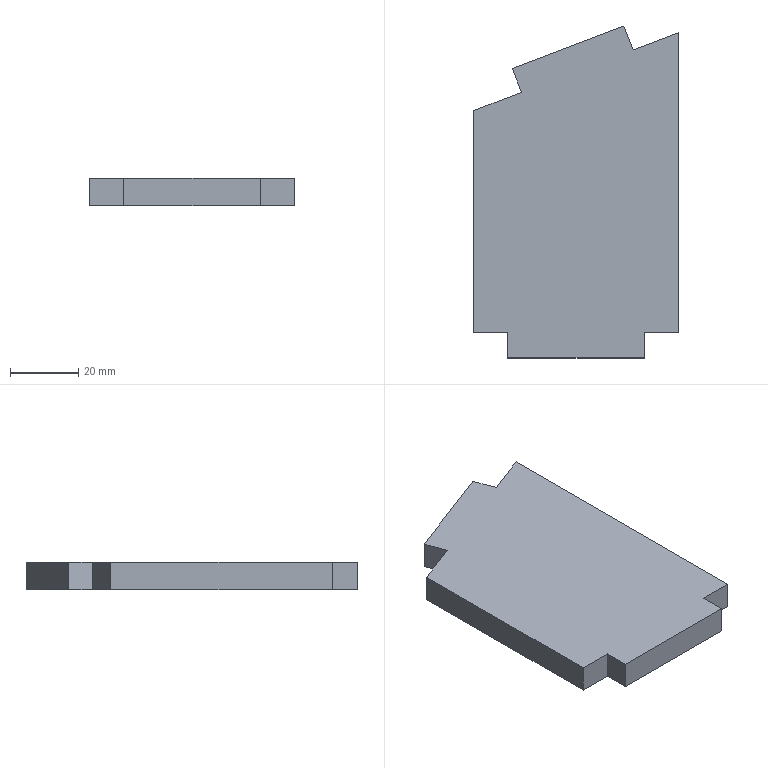Part | SolidWorks | features FlatPattern 1, SMBaseFlange 1, SheetMetal 1 | 1 solid | 14 faces | box 60 x 97.324 x 8 mm | volume 41194 mm3 | plane 14
STEP:
#1=CARTESIAN_POINT('',(134.399,-995.006,0.));
#2=VERTEX_POINT('',#1);
#3=CARTESIAN_POINT('',(144.399,-995.006,0.));
#4=VERTEX_POINT('',#3);
#5=CARTESIAN_POINT('',(144.399,-995.006,0.));
#6=DIRECTION('',(1.,0.,0.));
#7=VECTOR('',#6,1000.);
#8=LINE('',#5,#7);
#9=EDGE_CURVE('',#2,#4,#8,.T.);
#10=ORIENTED_EDGE('',*,*,#9,.F.);
#11=CARTESIAN_POINT('',(134.399,-995.006,-8.));
#12=VERTEX_POINT('',#11);
#13=CARTESIAN_POINT('',(134.399,-995.006,-8.));
#14=DIRECTION('',(0.,0.,1.));
#15=VECTOR('',#14,1000.);
#16=LINE('',#13,#15);
#17=EDGE_CURVE('',#12,#2,#16,.T.);
#18=ORIENTED_EDGE('',*,*,#17,.F.);
#19=CARTESIAN_POINT('',(144.399,-995.006,-8.));
#20=VERTEX_POINT('',#19);
#21=CARTESIAN_POINT('',(144.399,-995.006,-8.));
#22=DIRECTION('',(1.,0.,0.));
#23=VECTOR('',#22,1000.);
#24=LINE('',#21,#23);
#25=EDGE_CURVE('',#12,#20,#24,.T.);
#26=ORIENTED_EDGE('',*,*,#25,.T.);
#27=CARTESIAN_POINT('',(144.399,-995.006,-8.));
#28=DIRECTION('',(0.,0.,1.));
#29=VECTOR('',#28,1000.);
#30=LINE('',#27,#29);
#31=EDGE_CURVE('',#20,#4,#30,.T.);
#32=ORIENTED_EDGE('',*,*,#31,.T.);
#33=EDGE_LOOP('',(#10,#18,#26,#32));
#34=FACE_OUTER_BOUND('',#33,.T.);
#35=CARTESIAN_POINT('',(144.399,-995.006,-8.));
#36=DIRECTION('',(0.,-1.,0.));
#37=DIRECTION('',(0.,0.,-1.));
#38=AXIS2_PLACEMENT_3D('',#35,#36,#37);
#39=PLANE('',#38);
#40=ADVANCED_FACE('',(#34),#39,.T.);
#41=CARTESIAN_POINT('',(134.399,-929.986,0.));
#42=VERTEX_POINT('',#41);
#43=CARTESIAN_POINT('',(134.399,-995.006,0.));
#44=DIRECTION('',(0.,-1.,0.));
#45=VECTOR('',#44,1000.);
#46=LINE('',#43,#45);
#47=EDGE_CURVE('',#42,#2,#46,.T.);
#48=ORIENTED_EDGE('',*,*,#47,.F.);
#49=CARTESIAN_POINT('',(134.399,-929.986,-8.));
#50=VERTEX_POINT('',#49);
#51=CARTESIAN_POINT('',(134.399,-929.986,-8.));
#52=DIRECTION('',(0.,0.,1.));
#53=VECTOR('',#52,1000.);
#54=LINE('',#51,#53);
#55=EDGE_CURVE('',#50,#42,#54,.T.);
#56=ORIENTED_EDGE('',*,*,#55,.F.);
#57=CARTESIAN_POINT('',(134.399,-995.006,-8.));
#58=DIRECTION('',(0.,-1.,0.));
#59=VECTOR('',#58,1000.);
#60=LINE('',#57,#59);
#61=EDGE_CURVE('',#50,#12,#60,.T.);
#62=ORIENTED_EDGE('',*,*,#61,.T.);
#63=ORIENTED_EDGE('',*,*,#17,.T.);
#64=EDGE_LOOP('',(#48,#56,#62,#63));
#65=FACE_OUTER_BOUND('',#64,.T.);
#66=CARTESIAN_POINT('',(134.399,-995.006,-8.));
#67=DIRECTION('',(-1.,0.,0.));
#68=DIRECTION('',(0.,0.,1.));
#69=AXIS2_PLACEMENT_3D('',#66,#67,#68);
#70=PLANE('',#69);
#71=ADVANCED_FACE('',(#65),#70,.T.);
#72=CARTESIAN_POINT('',(148.417,-924.647,0.));
#73=VERTEX_POINT('',#72);
#74=CARTESIAN_POINT('',(134.399,-929.986,0.));
#75=DIRECTION('',(-0.9345,-0.3559,0.));
#76=VECTOR('',#75,1000.);
#77=LINE('',#74,#76);
#78=EDGE_CURVE('',#73,#42,#77,.T.);
#79=ORIENTED_EDGE('',*,*,#78,.F.);
#80=CARTESIAN_POINT('',(148.417,-924.647,-8.));
#81=VERTEX_POINT('',#80);
#82=CARTESIAN_POINT('',(148.417,-924.647,-8.));
#83=DIRECTION('',(0.,0.,1.));
#84=VECTOR('',#83,1000.);
#85=LINE('',#82,#84);
#86=EDGE_CURVE('',#81,#73,#85,.T.);
#87=ORIENTED_EDGE('',*,*,#86,.F.);
#88=CARTESIAN_POINT('',(134.399,-929.986,-8.));
#89=DIRECTION('',(-0.9345,-0.3559,0.));
#90=VECTOR('',#89,1000.);
#91=LINE('',#88,#90);
#92=EDGE_CURVE('',#81,#50,#91,.T.);
#93=ORIENTED_EDGE('',*,*,#92,.T.);
#94=ORIENTED_EDGE('',*,*,#55,.T.);
#95=EDGE_LOOP('',(#79,#87,#93,#94));
#96=FACE_OUTER_BOUND('',#95,.T.);
#97=CARTESIAN_POINT('',(134.399,-929.986,-8.));
#98=DIRECTION('',(-0.3559,0.9345,0.));
#99=DIRECTION('',(-0.9345,-0.3559,0.));
#100=AXIS2_PLACEMENT_3D('',#97,#98,#99);
#101=PLANE('',#100);
#102=ADVANCED_FACE('',(#96),#101,.T.);
#103=CARTESIAN_POINT('',(145.747,-917.639,0.));
#104=VERTEX_POINT('',#103);
#105=CARTESIAN_POINT('',(148.417,-924.647,0.));
#106=DIRECTION('',(0.3559,-0.9345,0.));
#107=VECTOR('',#106,1000.);
#108=LINE('',#105,#107);
#109=EDGE_CURVE('',#104,#73,#108,.T.);
#110=ORIENTED_EDGE('',*,*,#109,.F.);
#111=CARTESIAN_POINT('',(145.747,-917.639,-8.));
#112=VERTEX_POINT('',#111);
#113=CARTESIAN_POINT('',(145.747,-917.639,-8.));
#114=DIRECTION('',(0.,0.,1.));
#115=VECTOR('',#114,1000.);
#116=LINE('',#113,#115);
#117=EDGE_CURVE('',#112,#104,#116,.T.);
#118=ORIENTED_EDGE('',*,*,#117,.F.);
#119=CARTESIAN_POINT('',(148.417,-924.647,-8.));
#120=DIRECTION('',(0.3559,-0.9345,0.));
#121=VECTOR('',#120,1000.);
#122=LINE('',#119,#121);
#123=EDGE_CURVE('',#112,#81,#122,.T.);
#124=ORIENTED_EDGE('',*,*,#123,.T.);
#125=ORIENTED_EDGE('',*,*,#86,.T.);
#126=EDGE_LOOP('',(#110,#118,#124,#125));
#127=FACE_OUTER_BOUND('',#126,.T.);
#128=CARTESIAN_POINT('',(148.417,-924.647,-8.));
#129=DIRECTION('',(-0.9345,-0.3559,0.));
#130=DIRECTION('',(0.3559,-0.9345,0.));
#131=AXIS2_PLACEMENT_3D('',#128,#129,#130);
#132=PLANE('',#131);
#133=ADVANCED_FACE('',(#127),#132,.T.);
#134=CARTESIAN_POINT('',(178.455,-905.181,0.));
#135=VERTEX_POINT('',#134);
#136=CARTESIAN_POINT('',(145.747,-917.639,0.));
#137=DIRECTION('',(-0.9345,-0.3559,0.));
#138=VECTOR('',#137,1000.);
#139=LINE('',#136,#138);
#140=EDGE_CURVE('',#135,#104,#139,.T.);
#141=ORIENTED_EDGE('',*,*,#140,.F.);
#142=CARTESIAN_POINT('',(178.455,-905.181,-8.));
#143=VERTEX_POINT('',#142);
#144=CARTESIAN_POINT('',(178.455,-905.181,-8.));
#145=DIRECTION('',(0.,0.,1.));
#146=VECTOR('',#145,1000.);
#147=LINE('',#144,#146);
#148=EDGE_CURVE('',#143,#135,#147,.T.);
#149=ORIENTED_EDGE('',*,*,#148,.F.);
#150=CARTESIAN_POINT('',(145.747,-917.639,-8.));
#151=DIRECTION('',(-0.9345,-0.3559,0.));
#152=VECTOR('',#151,1000.);
#153=LINE('',#150,#152);
#154=EDGE_CURVE('',#143,#112,#153,.T.);
#155=ORIENTED_EDGE('',*,*,#154,.T.);
#156=ORIENTED_EDGE('',*,*,#117,.T.);
#157=EDGE_LOOP('',(#141,#149,#155,#156));
#158=FACE_OUTER_BOUND('',#157,.T.);
#159=CARTESIAN_POINT('',(145.747,-917.639,-8.));
#160=DIRECTION('',(-0.3559,0.9345,0.));
#161=DIRECTION('',(-0.9345,-0.3559,0.));
#162=AXIS2_PLACEMENT_3D('',#159,#160,#161);
#163=PLANE('',#162);
#164=ADVANCED_FACE('',(#158),#163,.T.);
#165=CARTESIAN_POINT('',(181.125,-912.19,0.));
#166=VERTEX_POINT('',#165);
#167=CARTESIAN_POINT('',(178.455,-905.181,0.));
#168=DIRECTION('',(-0.3559,0.9345,0.));
#169=VECTOR('',#168,1000.);
#170=LINE('',#167,#169);
#171=EDGE_CURVE('',#166,#135,#170,.T.);
#172=ORIENTED_EDGE('',*,*,#171,.F.);
#173=CARTESIAN_POINT('',(181.125,-912.19,-8.));
#174=VERTEX_POINT('',#173);
#175=CARTESIAN_POINT('',(181.125,-912.19,-8.));
#176=DIRECTION('',(0.,0.,1.));
#177=VECTOR('',#176,1000.);
#178=LINE('',#175,#177);
#179=EDGE_CURVE('',#174,#166,#178,.T.);
#180=ORIENTED_EDGE('',*,*,#179,.F.);
#181=CARTESIAN_POINT('',(178.455,-905.181,-8.));
#182=DIRECTION('',(-0.3559,0.9345,0.));
#183=VECTOR('',#182,1000.);
#184=LINE('',#181,#183);
#185=EDGE_CURVE('',#174,#143,#184,.T.);
#186=ORIENTED_EDGE('',*,*,#185,.T.);
#187=ORIENTED_EDGE('',*,*,#148,.T.);
#188=EDGE_LOOP('',(#172,#180,#186,#187));
#189=FACE_OUTER_BOUND('',#188,.T.);
#190=CARTESIAN_POINT('',(178.455,-905.181,-8.));
#191=DIRECTION('',(0.9345,0.3559,0.));
#192=DIRECTION('',(-0.3559,0.9345,0.));
#193=AXIS2_PLACEMENT_3D('',#190,#191,#192);
#194=PLANE('',#193);
#195=ADVANCED_FACE('',(#189),#194,.T.);
#196=CARTESIAN_POINT('',(194.399,-907.134,0.));
#197=VERTEX_POINT('',#196);
#198=CARTESIAN_POINT('',(181.125,-912.19,0.));
#199=DIRECTION('',(-0.9345,-0.3559,0.));
#200=VECTOR('',#199,1000.);
#201=LINE('',#198,#200);
#202=EDGE_CURVE('',#197,#166,#201,.T.);
#203=ORIENTED_EDGE('',*,*,#202,.F.);
#204=CARTESIAN_POINT('',(194.399,-907.134,-8.));
#205=VERTEX_POINT('',#204);
#206=CARTESIAN_POINT('',(194.399,-907.134,-8.));
#207=DIRECTION('',(0.,0.,1.));
#208=VECTOR('',#207,1000.);
#209=LINE('',#206,#208);
#210=EDGE_CURVE('',#205,#197,#209,.T.);
#211=ORIENTED_EDGE('',*,*,#210,.F.);
#212=CARTESIAN_POINT('',(181.125,-912.19,-8.));
#213=DIRECTION('',(-0.9345,-0.3559,0.));
#214=VECTOR('',#213,1000.);
#215=LINE('',#212,#214);
#216=EDGE_CURVE('',#205,#174,#215,.T.);
#217=ORIENTED_EDGE('',*,*,#216,.T.);
#218=ORIENTED_EDGE('',*,*,#179,.T.);
#219=EDGE_LOOP('',(#203,#211,#217,#218));
#220=FACE_OUTER_BOUND('',#219,.T.);
#221=CARTESIAN_POINT('',(181.125,-912.19,-8.));
#222=DIRECTION('',(-0.3559,0.9345,0.));
#223=DIRECTION('',(-0.9345,-0.3559,0.));
#224=AXIS2_PLACEMENT_3D('',#221,#222,#223);
#225=PLANE('',#224);
#226=ADVANCED_FACE('',(#220),#225,.T.);
#227=CARTESIAN_POINT('',(194.399,-995.006,0.));
#228=VERTEX_POINT('',#227);
#229=CARTESIAN_POINT('',(194.399,-907.134,0.));
#230=DIRECTION('',(0.,1.,0.));
#231=VECTOR('',#230,1000.);
#232=LINE('',#229,#231);
#233=EDGE_CURVE('',#228,#197,#232,.T.);
#234=ORIENTED_EDGE('',*,*,#233,.F.);
#235=CARTESIAN_POINT('',(194.399,-995.006,-8.));
#236=VERTEX_POINT('',#235);
#237=CARTESIAN_POINT('',(194.399,-995.006,-8.));
#238=DIRECTION('',(0.,0.,1.));
#239=VECTOR('',#238,1000.);
#240=LINE('',#237,#239);
#241=EDGE_CURVE('',#236,#228,#240,.T.);
#242=ORIENTED_EDGE('',*,*,#241,.F.);
#243=CARTESIAN_POINT('',(194.399,-907.134,-8.));
#244=DIRECTION('',(0.,1.,0.));
#245=VECTOR('',#244,1000.);
#246=LINE('',#243,#245);
#247=EDGE_CURVE('',#236,#205,#246,.T.);
#248=ORIENTED_EDGE('',*,*,#247,.T.);
#249=ORIENTED_EDGE('',*,*,#210,.T.);
#250=EDGE_LOOP('',(#234,#242,#248,#249));
#251=FACE_OUTER_BOUND('',#250,.T.);
#252=CARTESIAN_POINT('',(194.399,-907.134,-8.));
#253=DIRECTION('',(1.,0.,0.));
#254=DIRECTION('',(0.,0.,-1.));
#255=AXIS2_PLACEMENT_3D('',#252,#253,#254);
#256=PLANE('',#255);
#257=ADVANCED_FACE('',(#251),#256,.T.);
#258=CARTESIAN_POINT('',(184.399,-995.006,0.));
#259=VERTEX_POINT('',#258);
#260=CARTESIAN_POINT('',(194.399,-995.006,0.));
#261=DIRECTION('',(1.,0.,0.));
#262=VECTOR('',#261,1000.);
#263=LINE('',#260,#262);
#264=EDGE_CURVE('',#259,#228,#263,.T.);
#265=ORIENTED_EDGE('',*,*,#264,.F.);
#266=CARTESIAN_POINT('',(184.399,-995.006,-8.));
#267=VERTEX_POINT('',#266);
#268=CARTESIAN_POINT('',(184.399,-995.006,-8.));
#269=DIRECTION('',(0.,0.,1.));
#270=VECTOR('',#269,1000.);
#271=LINE('',#268,#270);
#272=EDGE_CURVE('',#267,#259,#271,.T.);
#273=ORIENTED_EDGE('',*,*,#272,.F.);
#274=CARTESIAN_POINT('',(194.399,-995.006,-8.));
#275=DIRECTION('',(1.,0.,0.));
#276=VECTOR('',#275,1000.);
#277=LINE('',#274,#276);
#278=EDGE_CURVE('',#267,#236,#277,.T.);
#279=ORIENTED_EDGE('',*,*,#278,.T.);
#280=ORIENTED_EDGE('',*,*,#241,.T.);
#281=EDGE_LOOP('',(#265,#273,#279,#280));
#282=FACE_OUTER_BOUND('',#281,.T.);
#283=CARTESIAN_POINT('',(194.399,-995.006,-8.));
#284=DIRECTION('',(0.,-1.,0.));
#285=DIRECTION('',(0.,0.,-1.));
#286=AXIS2_PLACEMENT_3D('',#283,#284,#285);
#287=PLANE('',#286);
#288=ADVANCED_FACE('',(#282),#287,.T.);
#289=CARTESIAN_POINT('',(184.399,-1002.506,0.));
#290=VERTEX_POINT('',#289);
#291=CARTESIAN_POINT('',(184.399,-1002.506,0.));
#292=DIRECTION('',(0.,1.,0.));
#293=VECTOR('',#292,1000.);
#294=LINE('',#291,#293);
#295=EDGE_CURVE('',#290,#259,#294,.T.);
#296=ORIENTED_EDGE('',*,*,#295,.F.);
#297=CARTESIAN_POINT('',(184.399,-1002.506,-8.));
#298=VERTEX_POINT('',#297);
#299=CARTESIAN_POINT('',(184.399,-1002.506,-8.));
#300=DIRECTION('',(0.,0.,1.));
#301=VECTOR('',#300,1000.);
#302=LINE('',#299,#301);
#303=EDGE_CURVE('',#298,#290,#302,.T.);
#304=ORIENTED_EDGE('',*,*,#303,.F.);
#305=CARTESIAN_POINT('',(184.399,-1002.506,-8.));
#306=DIRECTION('',(0.,1.,0.));
#307=VECTOR('',#306,1000.);
#308=LINE('',#305,#307);
#309=EDGE_CURVE('',#298,#267,#308,.T.);
#310=ORIENTED_EDGE('',*,*,#309,.T.);
#311=ORIENTED_EDGE('',*,*,#272,.T.);
#312=EDGE_LOOP('',(#296,#304,#310,#311));
#313=FACE_OUTER_BOUND('',#312,.T.);
#314=CARTESIAN_POINT('',(184.399,-1002.506,-8.));
#315=DIRECTION('',(1.,0.,0.));
#316=DIRECTION('',(0.,0.,-1.));
#317=AXIS2_PLACEMENT_3D('',#314,#315,#316);
#318=PLANE('',#317);
#319=ADVANCED_FACE('',(#313),#318,.T.);
#320=CARTESIAN_POINT('',(144.399,-1002.506,0.));
#321=VERTEX_POINT('',#320);
#322=CARTESIAN_POINT('',(144.399,-1002.506,0.));
#323=DIRECTION('',(1.,0.,0.));
#324=VECTOR('',#323,1000.);
#325=LINE('',#322,#324);
#326=EDGE_CURVE('',#321,#290,#325,.T.);
#327=ORIENTED_EDGE('',*,*,#326,.F.);
#328=CARTESIAN_POINT('',(144.399,-1002.506,-8.));
#329=VERTEX_POINT('',#328);
#330=CARTESIAN_POINT('',(144.399,-1002.506,-8.));
#331=DIRECTION('',(0.,0.,1.));
#332=VECTOR('',#331,1000.);
#333=LINE('',#330,#332);
#334=EDGE_CURVE('',#329,#321,#333,.T.);
#335=ORIENTED_EDGE('',*,*,#334,.F.);
#336=CARTESIAN_POINT('',(144.399,-1002.506,-8.));
#337=DIRECTION('',(1.,0.,0.));
#338=VECTOR('',#337,1000.);
#339=LINE('',#336,#338);
#340=EDGE_CURVE('',#329,#298,#339,.T.);
#341=ORIENTED_EDGE('',*,*,#340,.T.);
#342=ORIENTED_EDGE('',*,*,#303,.T.);
#343=EDGE_LOOP('',(#327,#335,#341,#342));
#344=FACE_OUTER_BOUND('',#343,.T.);
#345=CARTESIAN_POINT('',(144.399,-1002.506,-8.));
#346=DIRECTION('',(0.,-1.,0.));
#347=DIRECTION('',(0.,0.,-1.));
#348=AXIS2_PLACEMENT_3D('',#345,#346,#347);
#349=PLANE('',#348);
#350=ADVANCED_FACE('',(#344),#349,.T.);
#351=CARTESIAN_POINT('',(144.399,-995.006,0.));
#352=DIRECTION('',(0.,-1.,0.));
#353=VECTOR('',#352,1000.);
#354=LINE('',#351,#353);
#355=EDGE_CURVE('',#4,#321,#354,.T.);
#356=ORIENTED_EDGE('',*,*,#355,.F.);
#357=ORIENTED_EDGE('',*,*,#31,.F.);
#358=CARTESIAN_POINT('',(144.399,-995.006,-8.));
#359=DIRECTION('',(0.,-1.,0.));
#360=VECTOR('',#359,1000.);
#361=LINE('',#358,#360);
#362=EDGE_CURVE('',#20,#329,#361,.T.);
#363=ORIENTED_EDGE('',*,*,#362,.T.);
#364=ORIENTED_EDGE('',*,*,#334,.T.);
#365=EDGE_LOOP('',(#356,#357,#363,#364));
#366=FACE_OUTER_BOUND('',#365,.T.);
#367=CARTESIAN_POINT('',(144.399,-995.006,-8.));
#368=DIRECTION('',(-1.,0.,0.));
#369=DIRECTION('',(0.,-1.,0.));
#370=AXIS2_PLACEMENT_3D('',#367,#368,#369);
#371=PLANE('',#370);
#372=ADVANCED_FACE('',(#366),#371,.T.);
#373=ORIENTED_EDGE('',*,*,#25,.F.);
#374=ORIENTED_EDGE('',*,*,#61,.F.);
#375=ORIENTED_EDGE('',*,*,#92,.F.);
#376=ORIENTED_EDGE('',*,*,#123,.F.);
#377=ORIENTED_EDGE('',*,*,#154,.F.);
#378=ORIENTED_EDGE('',*,*,#185,.F.);
#379=ORIENTED_EDGE('',*,*,#216,.F.);
#380=ORIENTED_EDGE('',*,*,#247,.F.);
#381=ORIENTED_EDGE('',*,*,#278,.F.);
#382=ORIENTED_EDGE('',*,*,#309,.F.);
#383=ORIENTED_EDGE('',*,*,#340,.F.);
#384=ORIENTED_EDGE('',*,*,#362,.F.);
#385=EDGE_LOOP('',(#373,#374,#375,#376,#377,#378,#379,#380,#381,#382,#383,#384));
#386=FACE_OUTER_BOUND('',#385,.T.);
#387=CARTESIAN_POINT('',(0.,0.,-8.));
#388=DIRECTION('',(0.,0.,-1.));
#389=DIRECTION('',(-1.,0.,0.));
#390=AXIS2_PLACEMENT_3D('',#387,#388,#389);
#391=PLANE('',#390);
#392=ADVANCED_FACE('',(#386),#391,.T.);
#393=ORIENTED_EDGE('',*,*,#9,.T.);
#394=ORIENTED_EDGE('',*,*,#355,.T.);
#395=ORIENTED_EDGE('',*,*,#326,.T.);
#396=ORIENTED_EDGE('',*,*,#295,.T.);
#397=ORIENTED_EDGE('',*,*,#264,.T.);
#398=ORIENTED_EDGE('',*,*,#233,.T.);
#399=ORIENTED_EDGE('',*,*,#202,.T.);
#400=ORIENTED_EDGE('',*,*,#171,.T.);
#401=ORIENTED_EDGE('',*,*,#140,.T.);
#402=ORIENTED_EDGE('',*,*,#109,.T.);
#403=ORIENTED_EDGE('',*,*,#78,.T.);
#404=ORIENTED_EDGE('',*,*,#47,.T.);
#405=EDGE_LOOP('',(#393,#394,#395,#396,#397,#398,#399,#400,#401,#402,#403,#404));
#406=FACE_OUTER_BOUND('',#405,.T.);
#407=CARTESIAN_POINT('',(0.,0.,0.));
#408=DIRECTION('',(0.,0.,-1.));
#409=DIRECTION('',(-1.,0.,0.));
#410=AXIS2_PLACEMENT_3D('',#407,#408,#409);
#411=PLANE('',#410);
#412=ADVANCED_FACE('',(#406),#411,.F.);
#413=CLOSED_SHELL('',(#40,#71,#102,#133,#164,#195,#226,#257,#288,#319,#350,#372,#392,#412));
#414=MANIFOLD_SOLID_BREP('',#413);
#415=CARTESIAN_POINT('',(0.,0.,0.));
#416=DIRECTION('',(0.,0.,1.));
#417=DIRECTION('',(1.,0.,0.));
#418=AXIS2_PLACEMENT_3D('',#415,#416,#417);
#419=(LENGTH_UNIT()NAMED_UNIT(*)SI_UNIT(.MILLI.,.METRE.));
#420=UNCERTAINTY_MEASURE_WITH_UNIT(LENGTH_MEASURE(0.00001),#419,'','');
#421=(NAMED_UNIT(*)PLANE_ANGLE_UNIT()SI_UNIT($,.RADIAN.));
#422=(NAMED_UNIT(*)SI_UNIT($,.STERADIAN.)SOLID_ANGLE_UNIT());
#423=(GEOMETRIC_REPRESENTATION_CONTEXT(3)GLOBAL_UNCERTAINTY_ASSIGNED_CONTEXT((#420))GLOBAL_UNIT_ASSIGNED_CONTEXT((#419,#421,#422))REPRESENTATION_CONTEXT('',''));
#424=ADVANCED_BREP_SHAPE_REPRESENTATION('',(#414,#418),#423);